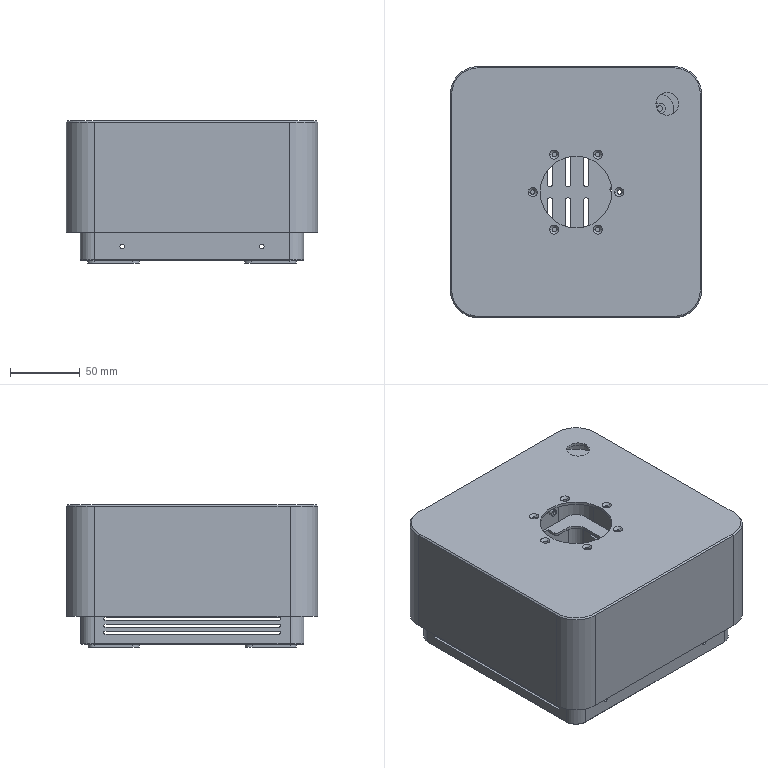Part | NX | features BREP 44 | 44 solids | 1182 faces | box 180 x 180.4 x 102 mm | volume 289321 mm3 | plane 507 | cylinder 382 | spline 273 | cone 20 | commonest cylinder face diameters 4 x115 2.5 x38 2 x31 3.2 x30 10 x27 8 x24